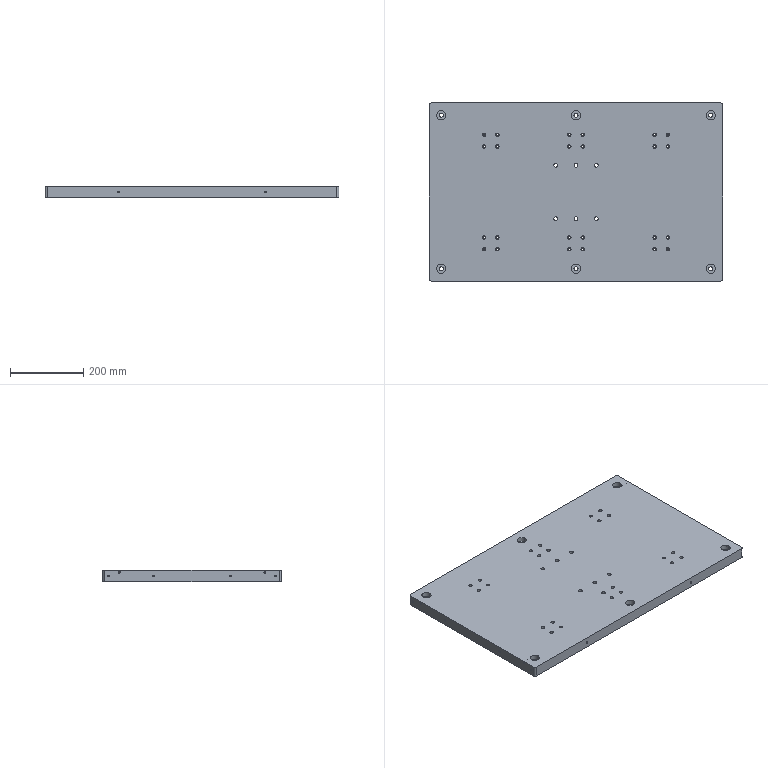NC program | Mastercam | posted with a generic post | part box 800 x 485 x 30 mm
Lines 3325 to 4968 of 13355:
N3520 T9 M6
N3530 G0 G90 G17 G54 X281.048 Y74.555 A0. S7000 M3
N3540 G43 H9 Z50. M8
N3550 Z1.
N3560 G1 Z-1.738 F600.
N3570 X280.896 Y75.543 F3000.
N3580 G3 X279.908 Y76.391 I-.988 J-.152
N3590 X279.756 Y76.379 I0. J-1.
N3600 G1 X273.1 Y75.355
N3610 Y69.122
N3620 G3 X274.1 Y68.122 I1. J0.
N3630 G1 X275.1
N3640 X281.048 Y74.555
N3650 Z-3.475 F600.
N3660 X280.896 Y75.543 F3000.
N3670 G3 X279.908 Y76.391 I-.988 J-.152
N3680 X279.756 Y76.379 I0. J-1.
N3690 G1 X273.1 Y75.355
N3700 Y69.122
N3710 G3 X274.1 Y68.122 I1. J0.
N3720 G1 X275.1
N3730 X281.048 Y74.555
N3740 Z-5.213 F600.
N3750 X280.896 Y75.543 F3000.
N3760 G3 X279.908 Y76.391 I-.988 J-.152
N3770 X279.756 Y76.379 I0. J-1.
N3780 G1 X273.1 Y75.355
N3790 Y69.122
N3800 G3 X274.1 Y68.122 I1. J0.
N3810 G1 X275.1
N3820 X281.048 Y74.555
N3830 Z-6.95 F600.
N3840 X280.896 Y75.543 F3000.
N3850 G3 X279.908 Y76.391 I-.988 J-.152
N3860 X279.756 Y76.379 I0. J-1.
N3870 G1 X273.1 Y75.355
N3880 Y69.122
N3890 G3 X274.1 Y68.122 I1. J0.
N3900 G1 X275.1
N3910 G0 Z50.
N3920 Y-75.399
N3930 Z1.
N3940 G1 Z-1.738 F600.
N3950 X274.1 F3000.
N3960 G3 X273.1 Y-76.399 I0. J-1.
N3970 G1 Y-83.4
N3980 X280.282
N3990 G3 X281.282 Y-82.4 I0. J1.
N4000 G1 Y-81.4
N4010 X275.1 Y-75.399
N4020 Z-3.475 F600.
N4030 X274.1 F3000.
N4040 G3 X273.1 Y-76.399 I0. J-1.
N4050 G1 Y-83.4
N4060 X280.282
N4070 G3 X281.282 Y-82.4 I0. J1.
N4080 G1 Y-81.4
N4090 X275.1 Y-75.399
N4100 Z-5.213 F600.
N4110 X274.1 F3000.
N4120 G3 X273.1 Y-76.399 I0. J-1.
N4130 G1 Y-83.4
N4140 X280.282
N4150 G3 X281.282 Y-82.4 I0. J1.
N4160 G1 Y-81.4
N4170 X275.1 Y-75.399
N4180 Z-6.95 F600.
N4190 X274.1 F3000.
N4200 G3 X273.1 Y-76.399 I0. J-1.
N4210 G1 Y-83.4
N4220 X280.282
N4230 G3 X281.282 Y-82.4 I0. J1.
N4240 G1 Y-81.4
N4250 G0 Z50.
N4260 X368.741
N4270 Z1.
N4280 G1 Z-1.738 F600.
N4290 Y-82.4 F3000.
N4300 G3 X369.741 Y-83.4 I1. J0.
N4310 G1 X376.9
N4320 Y-76.373
N4330 G3 X375.9 Y-75.373 I-1. J0.
N4340 G1 X374.9
N4350 X368.741 Y-81.4
N4360 Z-3.475 F600.
N4370 Y-82.4 F3000.
N4380 G3 X369.741 Y-83.4 I1. J0.
N4390 G1 X376.9
N4400 Y-76.373
N4410 G3 X375.9 Y-75.373 I-1. J0.
N4420 G1 X374.9
N4430 X368.741 Y-81.4
N4440 Z-5.213 F600.
N4450 Y-82.4 F3000.
N4460 G3 X369.741 Y-83.4 I1. J0.
N4470 G1 X376.9
N4480 Y-76.373
N4490 G3 X375.9 Y-75.373 I-1. J0.
N4500 G1 X374.9
N4510 X368.741 Y-81.4
N4520 Z-6.95 F600.
N4530 Y-82.4 F3000.
N4540 G3 X369.741 Y-83.4 I1. J0.
N4550 G1 X376.9
N4560 Y-76.373
N4570 G3 X375.9 Y-75.373 I-1. J0.
N4580 G1 X374.9
N4590 G0 Z50.
N4600 Y68.162
N4610 Z1.
N4620 G1 Z-1.738 F600.
N4630 X375.9 F3000.
N4640 G3 X376.9 Y69.162 I0. J1.
N4650 G1 Y75.355
N4660 X370.266 Y76.376
N4670 G3 X370.114 Y76.388 I-.152 J-.988
N4680 X369.126 Y75.54 I0. J-1.
N4690 G1 X368.974 Y74.551
N4700 X374.9 Y68.162
N4710 Z-3.475 F600.
N4720 X375.9 F3000.
N4730 G3 X376.9 Y69.162 I0. J1.
N4740 G1 Y75.355
N4750 X370.266 Y76.376
N4760 G3 X370.114 Y76.388 I-.152 J-.988
N4770 X369.126 Y75.54 I0. J-1.
N4780 G1 X368.974 Y74.551
N4790 X374.9 Y68.162
N4800 Z-5.213 F600.
N4810 X375.9 F3000.
N4820 G3 X376.9 Y69.162 I0. J1.
N4830 G1 Y75.355
N4840 X370.266 Y76.376
N4850 G3 X370.114 Y76.388 I-.152 J-.988
N4860 X369.126 Y75.54 I0. J-1.
N4870 G1 X368.974 Y74.551
N4880 X374.9 Y68.162
N4890 Z-6.95 F600.
N4900 X375.9 F3000.
N4910 G3 X376.9 Y69.162 I0. J1.
N4920 G1 Y75.355
N4930 X370.266 Y76.376
N4940 G3 X370.114 Y76.388 I-.152 J-.988
N4950 X369.126 Y75.54 I0. J-1.
N4960 G1 X368.974 Y74.551
N4970 G0 Z50.
N4980 X151.048 Y74.555
N4990 Z1.
N5000 G1 Z-1.738 F600.
N5010 X150.896 Y75.543 F3000.
N5020 G3 X149.908 Y76.391 I-.988 J-.152
N5030 X149.756 Y76.379 I0. J-1.
N5040 G1 X143.1 Y75.355
N5050 Y69.122
N5060 G3 X144.1 Y68.122 I1. J0.
N5070 G1 X145.1
N5080 X151.048 Y74.555
N5090 Z-3.475 F600.
N5100 X150.896 Y75.543 F3000.
N5110 G3 X149.908 Y76.391 I-.988 J-.152
N5120 X149.756 Y76.379 I0. J-1.
N5130 G1 X143.1 Y75.355
N5140 Y69.122
N5150 G3 X144.1 Y68.122 I1. J0.
N5160 G1 X145.1
N5170 X151.048 Y74.555
N5180 Z-5.213 F600.
N5190 X150.896 Y75.543 F3000.
N5200 G3 X149.908 Y76.391 I-.988 J-.152
N5210 X149.756 Y76.379 I0. J-1.
N5220 G1 X143.1 Y75.355
N5230 Y69.122
N5240 G3 X144.1 Y68.122 I1. J0.
N5250 G1 X145.1
N5260 X151.048 Y74.555
N5270 Z-6.95 F600.
N5280 X150.896 Y75.543 F3000.
N5290 G3 X149.908 Y76.391 I-.988 J-.152
N5300 X149.756 Y76.379 I0. J-1.
N5310 G1 X143.1 Y75.355
N5320 Y69.122
N5330 G3 X144.1 Y68.122 I1. J0.
N5340 G1 X145.1
N5350 G0 Z50.
N5360 Y-75.399
N5370 Z1.
N5380 G1 Z-1.738 F600.
N5390 X144.1 F3000.
N5400 G3 X143.1 Y-76.399 I0. J-1.
N5410 G1 Y-83.4
N5420 X150.282
N5430 G3 X151.282 Y-82.4 I0. J1.
N5440 G1 Y-81.4
N5450 X145.1 Y-75.399
N5460 Z-3.475 F600.
N5470 X144.1 F3000.
N5480 G3 X143.1 Y-76.399 I0. J-1.
N5490 G1 Y-83.4
N5500 X150.282
N5510 G3 X151.282 Y-82.4 I0. J1.
N5520 G1 Y-81.4
N5530 X145.1 Y-75.399
N5540 Z-5.213 F600.
N5550 X144.1 F3000.
N5560 G3 X143.1 Y-76.399 I0. J-1.
N5570 G1 Y-83.4
N5580 X150.282
N5590 G3 X151.282 Y-82.4 I0. J1.
N5600 G1 Y-81.4
N5610 X145.1 Y-75.399
N5620 Z-6.95 F600.
N5630 X144.1 F3000.
N5640 G3 X143.1 Y-76.399 I0. J-1.
N5650 G1 Y-83.4
N5660 X150.282
N5670 G3 X151.282 Y-82.4 I0. J1.
N5680 G1 Y-81.4
N5690 G0 Z50.
N5700 X238.694
N5710 Z1.
N5720 G1 Z-1.738 F600.
N5730 Y-82.4 F3000.
N5740 G3 X239.694 Y-83.4 I1. J0.
N5750 G1 X246.9
N5760 Y-76.373
N5770 G3 X245.9 Y-75.373 I-1. J0.
N5780 G1 X244.9
N5790 X238.694 Y-81.4
N5800 Z-3.475 F600.
N5810 Y-82.4 F3000.
N5820 G3 X239.694 Y-83.4 I1. J0.
N5830 G1 X246.9
N5840 Y-76.373
N5850 G3 X245.9 Y-75.373 I-1. J0.
N5860 G1 X244.9
N5870 X238.694 Y-81.4
N5880 Z-5.213 F600.
N5890 Y-82.4 F3000.
N5900 G3 X239.694 Y-83.4 I1. J0.
N5910 G1 X246.9
N5920 Y-76.373
N5930 G3 X245.9 Y-75.373 I-1. J0.
N5940 G1 X244.9
N5950 X238.694 Y-81.4
N5960 Z-6.95 F600.
N5970 Y-82.4 F3000.
N5980 G3 X239.694 Y-83.4 I1. J0.
N5990 G1 X246.9
N6000 Y-76.373
N6010 G3 X245.9 Y-75.373 I-1. J0.
N6020 G1 X244.9
N6030 G0 Z50.
N6040 Y68.163
N6050 Z1.
N6060 G1 Z-1.738 F600.
N6070 X245.9 F3000.
N6080 G3 X246.9 Y69.163 I0. J1.
N6090 G1 Y75.355
N6100 X240.266 Y76.376
N6110 G3 X240.114 Y76.388 I-.152 J-.988
N6120 X239.126 Y75.54 I0. J-1.
N6130 G1 X238.974 Y74.551
N6140 X244.9 Y68.163
N6150 Z-3.475 F600.
N6160 X245.9 F3000.
N6170 G3 X246.9 Y69.163 I0. J1.
N6180 G1 Y75.355
N6190 X240.266 Y76.376
N6200 G3 X240.114 Y76.388 I-.152 J-.988
N6210 X239.126 Y75.54 I0. J-1.
N6220 G1 X238.974 Y74.551
N6230 X244.9 Y68.163
N6240 Z-5.213 F600.
N6250 X245.9 F3000.
N6260 G3 X246.9 Y69.163 I0. J1.
N6270 G1 Y75.355
N6280 X240.266 Y76.376
N6290 G3 X240.114 Y76.388 I-.152 J-.988
N6300 X239.126 Y75.54 I0. J-1.
N6310 G1 X238.974 Y74.551
N6320 X244.9 Y68.163
N6330 Z-6.95 F600.
N6340 X245.9 F3000.
N6350 G3 X246.9 Y69.163 I0. J1.
N6360 G1 Y75.355
N6370 X240.266 Y76.376
N6380 G3 X240.114 Y76.388 I-.152 J-.988
N6390 X239.126 Y75.54 I0. J-1.
N6400 G1 X238.974 Y74.551
N6410 G0 Z50.
N6420 X21.048 Y74.555
N6430 Z1.
N6440 G1 Z-1.738 F600.
N6450 X20.896 Y75.543 F3000.
N6460 G3 X19.908 Y76.391 I-.988 J-.152
N6470 X19.756 Y76.379 I0. J-1.
N6480 G1 X13.1 Y75.355
N6490 Y69.122
N6500 G3 X14.1 Y68.122 I1. J0.
N6510 G1 X15.1
N6520 X21.048 Y74.555
N6530 Z-3.475 F600.
N6540 X20.896 Y75.543 F3000.
N6550 G3 X19.908 Y76.391 I-.988 J-.152
N6560 X19.756 Y76.379 I0. J-1.
N6570 G1 X13.1 Y75.355
N6580 Y69.122
N6590 G3 X14.1 Y68.122 I1. J0.
N6600 G1 X15.1
N6610 X21.048 Y74.555
N6620 Z-5.213 F600.
N6630 X20.896 Y75.543 F3000.
N6640 G3 X19.908 Y76.391 I-.988 J-.152
N6650 X19.756 Y76.379 I0. J-1.
N6660 G1 X13.1 Y75.355
N6670 Y69.122
N6680 G3 X14.1 Y68.122 I1. J0.
N6690 G1 X15.1
N6700 X21.048 Y74.555
N6710 Z-6.95 F600.
N6720 X20.896 Y75.543 F3000.
N6730 G3 X19.908 Y76.391 I-.988 J-.152
N6740 X19.756 Y76.379 I0. J-1.
N6750 G1 X13.1 Y75.355
N6760 Y69.122
N6770 G3 X14.1 Y68.122 I1. J0.
N6780 G1 X15.1
N6790 G0 Z50.
N6800 Y-75.399
N6810 Z1.
N6820 G1 Z-1.738 F600.
N6830 X14.1 F3000.
N6840 G3 X13.1 Y-76.399 I0. J-1.
N6850 G1 Y-83.4
N6860 X20.282
N6870 G3 X21.282 Y-82.4 I0. J1.
N6880 G1 Y-81.4
N6890 X15.1 Y-75.399
N6900 Z-3.475 F600.
N6910 X14.1 F3000.
N6920 G3 X13.1 Y-76.399 I0. J-1.
N6930 G1 Y-83.4
N6940 X20.282
N6950 G3 X21.282 Y-82.4 I0. J1.
N6960 G1 Y-81.4
N6970 X15.1 Y-75.399
N6980 Z-5.213 F600.
N6990 X14.1 F3000.
N7000 G3 X13.1 Y-76.399 I0. J-1.
N7010 G1 Y-83.4
N7020 X20.282
N7030 G3 X21.282 Y-82.4 I0. J1.
N7040 G1 Y-81.4
N7050 X15.1 Y-75.399
N7060 Z-6.95 F600.
N7070 X14.1 F3000.
N7080 G3 X13.1 Y-76.399 I0. J-1.
N7090 G1 Y-83.4
N7100 X20.282
N7110 G3 X21.282 Y-82.4 I0. J1.
N7120 G1 Y-81.4
N7130 G0 Z50.
N7140 X108.744
N7150 Z1.
N7160 G1 Z-1.738 F600.
N7170 Y-82.4 F3000.
N7180 G3 X109.744 Y-83.4 I1. J0.
N7190 G1 X116.9
N7200 Y-76.373
N7210 G3 X115.9 Y-75.373 I-1. J0.
N7220 G1 X114.9
N7230 X108.744 Y-81.4
N7240 Z-3.475 F600.
N7250 Y-82.4 F3000.
N7260 G3 X109.744 Y-83.4 I1. J0.
N7270 G1 X116.9
N7280 Y-76.373
N7290 G3 X115.9 Y-75.373 I-1. J0.
N7300 G1 X114.9
N7310 X108.744 Y-81.4
N7320 Z-5.213 F600.
N7330 Y-82.4 F3000.
N7340 G3 X109.744 Y-83.4 I1. J0.
N7350 G1 X116.9
N7360 Y-76.373
N7370 G3 X115.9 Y-75.373 I-1. J0.
N7380 G1 X114.9
N7390 X108.744 Y-81.4
N7400 Z-6.95 F600.
N7410 Y-82.4 F3000.
N7420 G3 X109.744 Y-83.4 I1. J0.
N7430 G1 X116.9
N7440 Y-76.373
N7450 G3 X115.9 Y-75.373 I-1. J0.
N7460 G1 X114.9
N7470 G0 Z50.
N7480 Y68.106
N7490 Z1.
N7500 G1 Z-1.738 F600.
N7510 X115.9 F3000.
N7520 G3 X116.9 Y69.106 I0. J1.
N7530 G1 Y75.355
N7540 X110.266 Y76.376
N7550 G3 X110.114 Y76.388 I-.152 J-.988
N7560 X109.126 Y75.54 I0. J-1.
N7570 G1 X108.974 Y74.551
N7580 X114.9 Y68.106
N7590 Z-3.475 F600.
N7600 X115.9 F3000.
N7610 G3 X116.9 Y69.106 I0. J1.
N7620 G1 Y75.355
N7630 X110.266 Y76.376
N7640 G3 X110.114 Y76.388 I-.152 J-.988
N7650 X109.126 Y75.54 I0. J-1.
N7660 G1 X108.974 Y74.551
N7670 X114.9 Y68.106
N7680 Z-5.213 F600.
N7690 X115.9 F3000.
N7700 G3 X116.9 Y69.106 I0. J1.
N7710 G1 Y75.355
N7720 X110.266 Y76.376
N7730 G3 X110.114 Y76.388 I-.152 J-.988
N7740 X109.126 Y75.54 I0. J-1.
N7750 G1 X108.974 Y74.551
N7760 X114.9 Y68.106
N7770 Z-6.95 F600.
N7780 X115.9 F3000.
N7790 G3 X116.9 Y69.106 I0. J1.
N7800 G1 Y75.355
N7810 X110.266 Y76.376
N7820 G3 X110.114 Y76.388 I-.152 J-.988
N7830 X109.126 Y75.54 I0. J-1.
N7840 G1 X108.974 Y74.551
N7850 G0 Z50.
N7860 X-238.952 Y74.555
N7870 Z1.
N7880 G1 Z-1.738 F600.
N7890 X-239.104 Y75.543 F3000.
N7900 G3 X-240.092 Y76.391 I-.988 J-.152
N7910 X-240.244 Y76.379 I0. J-1.
N7920 G1 X-246.9 Y75.355
N7930 Y69.122
N7940 G3 X-245.9 Y68.122 I1. J0.
N7950 G1 X-244.9
N7960 X-238.952 Y74.555
N7970 Z-3.475 F600.
N7980 X-239.104 Y75.543 F3000.
N7990 G3 X-240.092 Y76.391 I-.988 J-.152
N8000 X-240.244 Y76.379 I0. J-1.
N8010 G1 X-246.9 Y75.355
N8020 Y69.122
N8030 G3 X-245.9 Y68.122 I1. J0.
N8040 G1 X-244.9
N8050 X-238.952 Y74.555
N8060 Z-5.213 F600.
N8070 X-239.104 Y75.543 F3000.
N8080 G3 X-240.092 Y76.391 I-.988 J-.152
N8090 X-240.244 Y76.379 I0. J-1.
N8100 G1 X-246.9 Y75.355
N8110 Y69.122
N8120 G3 X-245.9 Y68.122 I1. J0.
N8130 G1 X-244.9
N8140 X-238.952 Y74.555
N8150 Z-6.95 F600.
N8160 X-239.104 Y75.543 F3000.
N8170 G3 X-240.092 Y76.391 I-.988 J-.152
N8180 X-240.244 Y76.379 I0. J-1.
N8190 G1 X-246.9 Y75.355
N8200 Y69.122
N8210 G3 X-245.9 Y68.122 I1. J0.
N8220 G1 X-244.9
N8230 G0 Z50.
N8240 Y-75.399
N8250 Z1.
N8260 G1 Z-1.738 F600.
N8270 X-245.9 F3000.
N8280 G3 X-246.9 Y-76.399 I0. J-1.
N8290 G1 Y-83.4
N8300 X-239.718
N8310 G3 X-238.718 Y-82.4 I0. J1.
N8320 G1 Y-81.4
N8330 X-244.9 Y-75.399
N8340 Z-3.475 F600.
N8350 X-245.9 F3000.
N8360 G3 X-246.9 Y-76.399 I0. J-1.
N8370 G1 Y-83.4
N8380 X-239.718
N8390 G3 X-238.718 Y-82.4 I0. J1.
N8400 G1 Y-81.4
N8410 X-244.9 Y-75.399
N8420 Z-5.213 F600.
N8430 X-245.9 F3000.
N8440 G3 X-246.9 Y-76.399 I0. J-1.
N8450 G1 Y-83.4
N8460 X-239.718
N8470 G3 X-238.718 Y-82.4 I0. J1.
N8480 G1 Y-81.4
N8490 X-244.9 Y-75.399
N8500 Z-6.95 F600.
N8510 X-245.9 F3000.
N8520 G3 X-246.9 Y-76.399 I0. J-1.
N8530 G1 Y-83.4
N8540 X-239.718
N8550 G3 X-238.718 Y-82.4 I0. J1.
N8560 G1 Y-81.4
N8570 G0 Z50.
N8580 X-151.306
N8590 Z1.
N8600 G1 Z-1.738 F600.
N8610 Y-82.4 F3000.
N8620 G3 X-150.306 Y-83.4 I1. J0.
N8630 G1 X-143.1
N8640 Y-76.373
N8650 G3 X-144.1 Y-75.373 I-1. J0.
N8660 G1 X-145.1
N8670 X-151.306 Y-81.4
N8680 Z-3.475 F600.
N8690 Y-82.4 F3000.
N8700 G3 X-150.306 Y-83.4 I1. J0.
N8710 G1 X-143.1
N8720 Y-76.373
N8730 G3 X-144.1 Y-75.373 I-1. J0.
N8740 G1 X-145.1
N8750 X-151.306 Y-81.4
N8760 Z-5.213 F600.
N8770 Y-82.4 F3000.
N8780 G3 X-150.306 Y-83.4 I1. J0.
N8790 G1 X-143.1
N8800 Y-76.373
N8810 G3 X-144.1 Y-75.373 I-1. J0.
N8820 G1 X-145.1
N8830 X-151.306 Y-81.4
N8840 Z-6.95 F600.
N8850 Y-82.4 F3000.
N8860 G3 X-150.306 Y-83.4 I1. J0.
N8870 G1 X-143.1
N8880 Y-76.373
N8890 G3 X-144.1 Y-75.373 I-1. J0.
N8900 G1 X-145.1
N8910 G0 Z50.
N8920 Y68.163
N8930 Z1.
N8940 G1 Z-1.738 F600.
N8950 X-144.1 F3000.
N8960 G3 X-143.1 Y69.163 I0. J1.
N8970 G1 Y75.355
N8980 X-149.734 Y76.376
N8990 G3 X-149.886 Y76.388 I-.152 J-.988
N9000 X-150.874 Y75.54 I0. J-1.
N9010 G1 X-151.026 Y74.551
N9020 X-145.1 Y68.163
N9030 Z-3.475 F600.
N9040 X-144.1 F3000.
N9050 G3 X-143.1 Y69.163 I0. J1.
N9060 G1 Y75.355
N9070 X-149.734 Y76.376
N9080 G3 X-149.886 Y76.388 I-.152 J-.988
N9090 X-150.874 Y75.54 I0. J-1.
N9100 G1 X-151.026 Y74.551
N9110 X-145.1 Y68.163
N9120 Z-5.213 F600.
N9130 X-144.1 F3000.
N9140 G3 X-143.1 Y69.163 I0. J1.
N9150 G1 Y75.355
N9160 X-149.734 Y76.376
N9170 G3 X-149.886 Y76.388 I-.152 J-.988
N9180 X-150.874 Y75.54 I0. J-1.
N9190 G1 X-151.026 Y74.551
N9200 X-145.1 Y68.163
N9210 Z-6.95 F600.
N9220 X-144.1 F3000.
N9230 G3 X-143.1 Y69.163 I0. J1.
N9240 G1 Y75.355
N9250 X-149.734 Y76.376
N9260 G3 X-149.886 Y76.388 I-.152 J-.988
N9270 X-150.874 Y75.54 I0. J-1.
N9280 G1 X-151.026 Y74.551
N9290 G0 Z50.
N9300 X-321.94 Y80.846
N9310 Z1.
N9320 G1 Z-1.738 F600.
N9330 X-321.788 Y81.834 F3000.
N9340 G3 X-321.776 Y81.986 I-.988 J.152
N9350 X-322.624 Y82.975 I-1. J0.
N9360 G1 X-325. Y83.34
N9370 X-328.29 Y82.834
N9380 G3 X-329.137 Y81.846 I.153 J-.988
N9390 X-329.126 Y81.693 I1. J0.
N9400 G1 X-328.974 Y80.705
N9410 X-321.94 Y80.846
N9420 Z-3.475 F600.
N9430 X-321.788 Y81.834 F3000.
N9440 G3 X-321.776 Y81.986 I-.988 J.152
N9450 X-322.624 Y82.975 I-1. J0.
N9460 G1 X-325. Y83.34
N9470 X-328.29 Y82.834
N9480 G3 X-329.137 Y81.846 I.153 J-.988
N9490 X-329.126 Y81.693 I1. J0.
N9500 G1 X-328.974 Y80.705
N9510 X-321.94 Y80.846
N9520 Z-5.213 F600.
N9530 X-321.788 Y81.834 F3000.
N9540 G3 X-321.776 Y81.986 I-.988 J.152
N9550 X-322.624 Y82.975 I-1. J0.
N9560 G1 X-325. Y83.34
N9570 X-328.29 Y82.834
N9580 G3 X-329.137 Y81.846 I.153 J-.988
N9590 X-329.126 Y81.693 I1. J0.
N9600 G1 X-328.974 Y80.705
N9610 X-321.94 Y80.846
N9620 Z-6.95 F600.
N9630 X-321.788 Y81.834 F3000.
N9640 G3 X-321.776 Y81.986 I-.988 J.152
N9650 X-322.624 Y82.975 I-1. J0.
N9660 G1 X-325. Y83.34
N9670 X-328.29 Y82.834
N9680 G3 X-329.137 Y81.846 I.153 J-.988
N9690 X-329.126 Y81.693 I1. J0.
N9700 G1 X-328.974 Y80.705
N9710 G0 Z50.
N9720 X-368.952 Y74.555
N9730 Z1.
N9740 G1 Z-1.738 F600.
N9750 X-369.104 Y75.543 F3000.
N9760 G3 X-370.092 Y76.391 I-.988 J-.152
N9770 X-370.244 Y76.379 I0. J-1.
N9780 G1 X-376.9 Y75.355
N9790 Y69.122
N9800 G3 X-375.9 Y68.122 I1. J0.
N9810 G1 X-374.9
N9820 X-368.952 Y74.555
N9830 Z-3.475 F600.
N9840 X-369.104 Y75.543 F3000.
N9850 G3 X-370.092 Y76.391 I-.988 J-.152
N9860 X-370.244 Y76.379 I0. J-1.
N9870 G1 X-376.9 Y75.355
N9880 Y69.122
N9890 G3 X-375.9 Y68.122 I1. J0.
N9900 G1 X-374.9
N9910 X-368.952 Y74.555
N9920 Z-5.213 F600.
N9930 X-369.104 Y75.543 F3000.
N9940 G3 X-370.092 Y76.391 I-.988 J-.152
N9950 X-370.244 Y76.379 I0. J-1.
N9960 G1 X-376.9 Y75.355
N9970 Y69.122
N9980 G3 X-375.9 Y68.122 I1. J0.
N9990 G1 X-374.9
N100 X-368.952 Y74.555
N110 Z-6.95 F600.
N120 X-369.104 Y75.543 F3000.
N130 G3 X-370.092 Y76.391 I-.988 J-.152
N140 X-370.244 Y76.379 I0. J-1.
N150 G1 X-376.9 Y75.355
N160 Y69.122
N170 G3 X-375.9 Y68.122 I1. J0.
N180 G1 X-374.9
N190 G0 Z50.
N200 Y-75.399
N210 Z1.
N220 G1 Z-1.738 F600.
N230 X-375.9 F3000.
N240 G3 X-376.9 Y-76.399 I0. J-1.
N250 G1 Y-83.4
N260 X-369.718
N270 G3 X-368.718 Y-82.4 I0. J1.
N280 G1 Y-81.4
N290 X-374.9 Y-75.399
N300 Z-3.475 F600.
N310 X-375.9 F3000.
N320 G3 X-376.9 Y-76.399 I0. J-1.
N330 G1 Y-83.4
N340 X-369.718
N350 G3 X-368.718 Y-82.4 I0. J1.
N360 G1 Y-81.4
N370 X-374.9 Y-75.399
N380 Z-5.213 F600.
N390 X-375.9 F3000.
N400 G3 X-376.9 Y-76.399 I0. J-1.
N410 G1 Y-83.4
N420 X-369.718
N430 G3 X-368.718 Y-82.4 I0. J1.
N440 G1 Y-81.4
N450 X-374.9 Y-75.399
N460 Z-6.95 F600.
N470 X-375.9 F3000.
N480 G3 X-376.9 Y-76.399 I0. J-1.
N490 G1 Y-83.4
N500 X-369.718
N510 G3 X-368.718 Y-82.4 I0. J1.
N520 G1 Y-81.4
N530 G0 Z50.
N540 X-281.256
N550 Z1.
N560 G1 Z-1.738 F600.
N570 Y-82.4 F3000.
N580 G3 X-280.256 Y-83.4 I1. J0.
N590 G1 X-273.1
N600 Y-76.373
N610 G3 X-274.1 Y-75.373 I-1. J0.
N620 G1 X-275.1
N630 X-281.256 Y-81.4
N640 Z-3.475 F600.
N650 Y-82.4 F3000.
N660 G3 X-280.256 Y-83.4 I1. J0.
N670 G1 X-273.1
N680 Y-76.373
N690 G3 X-274.1 Y-75.373 I-1. J0.
N700 G1 X-275.1
N710 X-281.256 Y-81.4
N720 Z-5.213 F600.
N730 Y-82.4 F3000.
N740 G3 X-280.256 Y-83.4 I1. J0.
N750 G1 X-273.1
N760 Y-76.373
N770 G3 X-274.1 Y-75.373 I-1. J0.
N780 G1 X-275.1
N790 X-281.256 Y-81.4
N800 Z-6.95 F600.
N810 Y-82.4 F3000.
N820 G3 X-280.256 Y-83.4 I1. J0.
N830 G1 X-273.1
N840 Y-76.373
N850 G3 X-274.1 Y-75.373 I-1. J0.
N860 G1 X-275.1
N870 G0 Z50.
N880 Y68.122
N890 Z1.
N900 G1 Z-1.738 F600.
N910 X-274.1 F3000.
N920 G3 X-273.1 Y69.122 I0. J1.
N930 G1 Y75.355
N940 X-279.734 Y76.376
N950 G3 X-279.886 Y76.388 I-.152 J-.988
N960 X-280.874 Y75.54 I0. J-1.
N970 G1 X-281.026 Y74.551
N980 X-275.1 Y68.122
N990 Z-3.475 F600.
N1000 X-274.1 F3000.
N1010 G3 X-273.1 Y69.122 I0. J1.
N1020 G1 Y75.355
N1030 X-279.734 Y76.376
N1040 G3 X-279.886 Y76.388 I-.152 J-.988
N1050 X-280.874 Y75.54 I0. J-1.
N1060 G1 X-281.026 Y74.551
N1070 X-275.1 Y68.122
N1080 Z-5.213 F600.
N1090 X-274.1 F3000.
N1100 G3 X-273.1 Y69.122 I0. J1.
N1110 G1 Y75.355
N1120 X-279.734 Y76.376
N1130 G3 X-279.886 Y76.388 I-.152 J-.988
N1140 X-280.874 Y75.54 I0. J-1.
N1150 G1 X-281.026 Y74.551
N1160 X-275.1 Y68.122
N1170 Z-6.95 F600.
N1180 X-274.1 F3000.
N1190 G3 X-273.1 Y69.122 I0. J1.
N1200 G1 Y75.355
N1210 X-279.734 Y76.376
N1220 G3 X-279.886 Y76.388 I-.152 J-.988
N1230 X-280.874 Y75.54 I0. J-1.
N1240 G1 X-281.026 Y74.551
N1250 G0 Z50.
N1260 X-108.952 Y74.555
N1270 Z1.
N1280 G1 Z-1.738 F600.
N1290 X-109.104 Y75.543 F3000.
N1300 G3 X-110.092 Y76.391 I-.988 J-.152
N1310 X-110.244 Y76.379 I0. J-1.
N1320 G1 X-116.9 Y75.355
N1330 Y69.122
N1340 G3 X-115.9 Y68.122 I1. J0.
N1350 G1 X-114.9
N1360 X-108.952 Y74.555
N1370 Z-3.475 F600.
N1380 X-109.104 Y75.543 F3000.
N1390 G3 X-110.092 Y76.391 I-.988 J-.152
N1400 X-110.244 Y76.379 I0. J-1.
N1410 G1 X-116.9 Y75.355
N1420 Y69.122
N1430 G3 X-115.9 Y68.122 I1. J0.
N1440 G1 X-114.9
N1450 X-108.952 Y74.555
N1460 Z-5.213 F600.
N1470 X-109.104 Y75.543 F3000.
N1480 G3 X-110.092 Y76.391 I-.988 J-.152
N1490 X-110.244 Y76.379 I0. J-1.
N1500 G1 X-116.9 Y75.355
N1510 Y69.122
N1520 G3 X-115.9 Y68.122 I1. J0.
N1530 G1 X-114.9
N1540 X-108.952 Y74.555
N1550 Z-6.95 F600.
N1560 X-109.104 Y75.543 F3000.
N1570 G3 X-110.092 Y76.391 I-.988 J-.152
N1580 X-110.244 Y76.379 I0. J-1.
N1590 G1 X-116.9 Y75.355
N1600 Y69.122
N1610 G3 X-115.9 Y68.122 I1. J0.
N1620 G1 X-114.9
N1630 G0 Z50.
N1640 Y-75.399
N1650 Z1.
N1660 G1 Z-1.738 F600.
N1670 X-115.9 F3000.
N1680 G3 X-116.9 Y-76.399 I0. J-1.
N1690 G1 Y-83.4
N1700 X-109.718
N1710 G3 X-108.718 Y-82.4 I0. J1.
N1720 G1 Y-81.4
N1730 X-114.9 Y-75.399
N1740 Z-3.475 F600.
N1750 X-115.9 F3000.
N1760 G3 X-116.9 Y-76.399 I0. J-1.
N1770 G1 Y-83.4
N1780 X-109.718
N1790 G3 X-108.718 Y-82.4 I0. J1.
N1800 G1 Y-81.4
N1810 X-114.9 Y-75.399
N1820 Z-5.213 F600.
N1830 X-115.9 F3000.
N1840 G3 X-116.9 Y-76.399 I0. J-1.
N1850 G1 Y-83.4
N1860 X-109.718
N1870 G3 X-108.718 Y-82.4 I0. J1.
N1880 G1 Y-81.4
N1890 X-114.9 Y-75.399
N1900 Z-6.95 F600.
N1910 X-115.9 F3000.
N1920 G3 X-116.9 Y-76.399 I0. J-1.
N1930 G1 Y-83.4
N1940 X-109.718
N1950 G3 X-108.718 Y-82.4 I0. J1.
N1960 G1 Y-81.4
N1970 G0 Z50.
N1980 X-21.256
N1990 Z1.
N2000 G1 Z-1.738 F600.
N2010 Y-82.4 F3000.
N2020 G3 X-20.256 Y-83.4 I1. J0.
N2030 G1 X-13.1
N2040 Y-76.373
N2050 G3 X-14.1 Y-75.373 I-1. J0.
N2060 G1 X-15.1
N2070 X-21.256 Y-81.4
N2080 Z-3.475 F600.
N2090 Y-82.4 F3000.
N2100 G3 X-20.256 Y-83.4 I1. J0.
N2110 G1 X-13.1
N2120 Y-76.373
N2130 G3 X-14.1 Y-75.373 I-1. J0.
N2140 G1 X-15.1
N2150 X-21.256 Y-81.4
N2160 Z-5.213 F600.
N2170 Y-82.4 F3000.
N2180 G3 X-20.256 Y-83.4 I1. J0.
N2190 G1 X-13.1
N2200 Y-76.373
N2210 G3 X-14.1 Y-75.373 I-1. J0.
N2220 G1 X-15.1
N2230 X-21.256 Y-81.4
N2240 Z-6.95 F600.
N2250 Y-82.4 F3000.
N2260 G3 X-20.256 Y-83.4 I1. J0.
N2270 G1 X-13.1
N2280 Y-76.373
N2290 G3 X-14.1 Y-75.373 I-1. J0.
N2300 G1 X-15.1
N2310 G0 Z50.
N2320 Y68.122
N2330 Z1.
N2340 G1 Z-1.738 F600.
N2350 X-14.1 F3000.
N2360 G3 X-13.1 Y69.122 I0. J1.
N2370 G1 Y75.355
N2380 X-19.734 Y76.376
N2390 G3 X-19.886 Y76.388 I-.152 J-.988
N2400 X-20.874 Y75.54 I0. J-1.
N2410 G1 X-21.026 Y74.551
N2420 X-15.1 Y68.122
N2430 Z-3.475 F600.
N2440 X-14.1 F3000.
N2450 G3 X-13.1 Y69.122 I0. J1.
N2460 G1 Y75.355
N2470 X-19.734 Y76.376
N2480 G3 X-19.886 Y76.388 I-.152 J-.988
N2490 X-20.874 Y75.54 I0. J-1.
N2500 G1 X-21.026 Y74.551
N2510 X-15.1 Y68.122
N2520 Z-5.213 F600.
N2530 X-14.1 F3000.
N2540 G3 X-13.1 Y69.122 I0. J1.
N2550 G1 Y75.355
N2560 X-19.734 Y76.376
N2570 G3 X-19.886 Y76.388 I-.152 J-.988
N2580 X-20.874 Y75.54 I0. J-1.
N2590 G1 X-21.026 Y74.551
N2600 X-15.1 Y68.122
N2610 Z-6.95 F600.
N2620 X-14.1 F3000.
N2630 G3 X-13.1 Y69.122 I0. J1.
N2640 G1 Y75.355
N2650 X-19.734 Y76.376
N2660 G3 X-19.886 Y76.388 I-.152 J-.988
N2670 X-20.874 Y75.54 I0. J-1.
N2680 G1 X-21.026 Y74.551
N2690 G0 Z50.
N2700 X-61.94 Y80.846
N2710 Z1.
N2720 G1 Z-1.738 F600.
N2730 X-61.788 Y81.834 F3000.
N2740 G3 X-61.776 Y81.986 I-.988 J.152
N2750 X-62.624 Y82.975 I-1. J0.
N2760 G1 X-65. Y83.34
N2770 X-68.29 Y82.834
N2780 G3 X-69.137 Y81.846 I.153 J-.988
N2790 X-69.126 Y81.693 I1. J0.
N2800 G1 X-68.974 Y80.705
N2810 X-61.94 Y80.846
N2820 Z-3.475 F600.
N2830 X-61.788 Y81.834 F3000.
N2840 G3 X-61.776 Y81.986 I-.988 J.152
N2850 X-62.624 Y82.975 I-1. J0.
N2860 G1 X-65. Y83.34
N2870 X-68.29 Y82.834
N2880 G3 X-69.137 Y81.846 I.153 J-.988
N2890 X-69.126 Y81.693 I1. J0.
N2900 G1 X-68.974 Y80.705
N2910 X-61.94 Y80.846
N2920 Z-5.213 F600.
N2930 X-61.788 Y81.834 F3000.
N2940 G3 X-61.776 Y81.986 I-.988 J.152
N2950 X-62.624 Y82.975 I-1. J0.
N2960 G1 X-65. Y83.34
N2970 X-68.29 Y82.834
N2980 G3 X-69.137 Y81.846 I.153 J-.988
N2990 X-69.126 Y81.693 I1. J0.
N3000 G1 X-68.974 Y80.705
N3010 X-61.94 Y80.846
N3020 Z-6.95 F600.
N3030 X-61.788 Y81.834 F3000.
N3040 G3 X-61.776 Y81.986 I-.988 J.152
N3050 X-62.624 Y82.975 I-1. J0.
N3060 G1 X-65. Y83.34
N3070 X-68.29 Y82.834
N3080 G3 X-69.137 Y81.846 I.153 J-.988
N3090 X-69.126 Y81.693 I1. J0.
N3100 G1 X-68.974 Y80.705
N3110 G0 Z50.
N3120 M5
N3130 G91 G28 Z0. M9
N3140 A0.
N3150 M01
N3160 T10 M6
N3170 G0 G90 G17 G54 X325. Y-7.851 A0. S7000 M3
N3180 G43 H10 Z50. M8
N3190 Z-6.
N3200 G1 Z-6.708 F600.
N3210 Y-2.351 Z-6.854 F1000.
N3220 Y-.335 Z-6.908
N3230 Y3.149 Z-7.
N3240 Y30.83
N3250 Y-31.5
N3260 Y-.335
N3270 Y3.149
N3280 G2 X325.805 Y4.155 I1.031 J0.
N3290 G1 X330.615 Y5.236
N3300 G3 X331.42 Y6.242 I-.226 J1.006
N3310 G1 Y36.337
N3320 X325. Y37.325
N3330 X318.58 Y36.337
N3340 Y-37.92
N3350 X331.42
N3360 Y-.335
N3370 Y6.242
N3380 G2 X332.229 Y7.249 I1.031 J0.
N3390 G1 X337.122 Y8.329
N3400 G3 X337.931 Y9.336 I-.222 J1.007
N3410 G1 Y41.923
N3420 X325. Y43.913
N3430 X312.069 Y41.923
N3440 Y-44.431
N3450 X337.931
N3460 Y-.335
N3470 Y9.336
N3480 G2 X338.74 Y10.343 I1.031 J0.
N3490 G1 X343.634 Y11.423
N3500 G3 X344.443 Y12.43 I-.223 J1.007
N3510 G1 Y47.51
N3520 X325. Y50.501
N3530 X305.557 Y47.51
N3540 Y-50.943
N3550 X344.443
N3560 Y-.335
N3570 Y12.43
N3580 G2 X345.252 Y13.437 I1.031 J0.
N3590 G1 X350.145 Y14.517
N3600 G3 X350.954 Y15.524 I-.222 J1.007
N3610 G1 Y53.096
N3620 X325. Y57.089
N3630 X299.046 Y53.096
N3640 Y-57.454
N3650 X350.954
N3660 Y-.335
N3670 Y15.524
N3680 G2 X351.763 Y16.531 I1.031 J0.
N3690 G1 X356.657 Y17.61
N3700 G3 X357.466 Y18.617 I-.223 J1.007
N3710 G1 Y58.682
N3720 X325. Y63.677
N3730 X292.534 Y58.682
N3740 Y-63.966
N3750 X357.466
N3760 Y-.335
N3770 Y18.617
N3780 G2 X358.275 Y19.624 I1.031 J0.
N3790 G1 X363.168 Y20.704
N3800 G3 X363.977 Y21.711 I-.222 J1.007
N3810 G1 Y64.269
N3820 X325. Y70.265
N3830 X286.023 Y64.269
N3840 Y-70.477
N3850 X363.977
N3860 Y-.335
N3870 Y21.711
N3880 G2 X364.786 Y22.718 I1.031 J0.
N3890 G1 X369.679 Y23.798
N3900 G3 X370.488 Y24.805 I-.222 J1.007
N3910 G1 Y69.855
N3920 X325. Y76.853
N3930 X279.512 Y69.855
N3940 Y-76.988
N3950 X370.488
N3960 Y-.335
N3970 Y24.805
N3980 G2 X371.297 Y25.812 I1.032 J0.
N3990 G1 X376.185 Y26.893
N4000 G3 X376.993 Y27.9 I-.223 J1.007
N4010 G1 X376.982 Y75.424
N4020 X325. Y83.427
N4030 X273.018 Y75.424
N4040 X273. Y75.084
N4050 Y-82.902
N4060 X273.022 Y-83.478
N4070 X273.523 Y-83.5
N4080 X376.477
N4090 X376.978 Y-83.478
N4100 X377. Y-82.902
N4110 Y-.335
N4120 X376.993 Y27.9
N4130 G0 Z50.
N4140 X195. Y-7.851
N4150 Z-6.
N4160 G1 Z-6.708 F600.
N4170 Y-2.351 Z-6.854 F1000.
N4180 Y-.335 Z-6.908
N4190 Y3.149 Z-7.
N4200 Y30.83
N4210 Y-31.5
N4220 Y-.335
N4230 Y3.149
N4240 G2 X195.805 Y4.155 I1.031 J0.
N4250 G1 X200.615 Y5.236
N4260 G3 X201.42 Y6.242 I-.226 J1.006
N4270 G1 Y36.337
N4280 X195. Y37.325
N4290 X188.58 Y36.337
N4300 Y-37.92
N4310 X201.42
N4320 Y-.335
N4330 Y6.242
N4340 G2 X202.229 Y7.249 I1.031 J0.
N4350 G1 X207.122 Y8.329
N4360 G3 X207.931 Y9.336 I-.222 J1.007
N4370 G1 Y41.923
N4380 X195. Y43.913
N4390 X182.069 Y41.923
N4400 Y-44.431
N4410 X207.931
N4420 Y-.335
N4430 Y9.336
N4440 G2 X208.74 Y10.343 I1.031 J0.
N4450 G1 X213.634 Y11.423
N4460 G3 X214.443 Y12.43 I-.223 J1.007
N4470 G1 Y47.51
N4480 X195. Y50.501
N4490 X175.557 Y47.51
N4500 Y-50.943
N4510 X214.443
N4520 Y-.335
N4530 Y12.43
N4540 G2 X215.252 Y13.437 I1.031 J0.
N4550 G1 X220.145 Y14.517
N4560 G3 X220.954 Y15.524 I-.222 J1.007
N4570 G1 Y53.096
N4580 X195. Y57.089
N4590 X169.046 Y53.096
N4600 Y-57.454
N4610 X220.954
N4620 Y-.335
N4630 Y15.524
N4640 G2 X221.763 Y16.531 I1.031 J0.
N4650 G1 X226.657 Y17.61
N4660 G3 X227.466 Y18.617 I-.223 J1.007
N4670 G1 Y58.682
N4680 X195. Y63.677
N4690 X162.534 Y58.682
N4700 Y-63.966
N4710 X227.466
N4720 Y-.335
N4730 Y18.617
N4740 G2 X228.275 Y19.624 I1.031 J0.
N4750 G1 X233.168 Y20.704
N4760 G3 X233.977 Y21.711 I-.222 J1.007
N4770 G1 Y64.269
N4780 X195. Y70.265
N4790 X156.023 Y64.269
N4800 Y-70.477
N4810 X233.977
N4820 Y-.335
N4830 Y21.711
N4840 G2 X234.786 Y22.718 I1.031 J0.
N4850 G1 X239.679 Y23.798
N4860 G3 X240.488 Y24.805 I-.222 J1.007
N4870 G1 Y69.855
N4880 X195. Y76.853
N4890 X149.512 Y69.855
N4900 Y-76.988
N4910 X240.488
N4920 Y-.335
N4930 Y24.805
N4940 G2 X241.297 Y25.812 I1.032 J0.
N4950 G1 X246.185 Y26.893
N4960 G3 X246.993 Y27.9 I-.223 J1.007
N4970 G1 X246.982 Y75.424
N4980 X195. Y83.427
N4990 X143.018 Y75.424
N5000 X143. Y75.084
N5010 Y-82.902
N5020 X143.022 Y-83.478
N5030 X143.523 Y-83.5
N5040 X246.477
N5050 X246.978 Y-83.478
N5060 X247. Y-82.902
N5070 Y-.335
N5080 X246.993 Y27.9
N5090 G0 Z50.
N5100 X65. Y-7.851
N5110 Z-6.
N5120 G1 Z-6.708 F600.
N5130 Y-2.351 Z-6.854 F1000.
N5140 Y-.335 Z-6.908
N5150 Y3.149 Z-7.
N5160 Y30.83
N5170 Y-31.5
N5180 Y-.335
N5190 Y3.149
N5200 G2 X65.805 Y4.155 I1.031 J0.
N5210 G1 X70.615 Y5.236
N5220 G3 X71.42 Y6.242 I-.226 J1.006
N5230 G1 Y36.337
N5240 X65. Y37.325
N5250 X58.58 Y36.337
N5260 Y-37.92
N5270 X71.42
N5280 Y-.335
N5290 Y6.242
N5300 G2 X72.229 Y7.249 I1.031 J0.
N5310 G1 X77.122 Y8.329
N5320 G3 X77.931 Y9.336 I-.222 J1.007
N5330 G1 Y41.923
N5340 X65. Y43.913
N5350 X52.069 Y41.923
N5360 Y-44.431
N5370 X77.931
N5380 Y-.335
N5390 Y9.336
N5400 G2 X78.74 Y10.343 I1.031 J0.
N5410 G1 X83.634 Y11.423
N5420 G3 X84.443 Y12.43 I-.223 J1.007
N5430 G1 Y47.51
N5440 X65. Y50.501
N5450 X45.557 Y47.51
N5460 Y-50.943
N5470 X84.443
N5480 Y-.335
N5490 Y12.43
N5500 G2 X85.252 Y13.437 I1.031 J0.
N5510 G1 X90.145 Y14.517
N5520 G3 X90.954 Y15.524 I-.222 J1.007
N5530 G1 Y53.096
N5540 X65. Y57.089
N5550 X39.046 Y53.096
N5560 Y-57.454
N5570 X90.954
N5580 Y-.335
N5590 Y15.524
N5600 G2 X91.763 Y16.531 I1.031 J0.
N5610 G1 X96.657 Y17.61
N5620 G3 X97.466 Y18.617 I-.223 J1.007
N5630 G1 Y58.682
N5640 X65. Y63.677
N5650 X32.534 Y58.682
N5660 Y-63.966
N5670 X97.466
N5680 Y-.335
N5690 Y18.617
N5700 G2 X98.275 Y19.624 I1.031 J0.
N5710 G1 X103.168 Y20.704
N5720 G3 X103.977 Y21.711 I-.222 J1.007
N5730 G1 Y64.269
N5740 X65. Y70.265
N5750 X26.023 Y64.269
N5760 Y-70.477
N5770 X103.977
N5780 Y-.335
N5790 Y21.711
N5800 G2 X104.786 Y22.718 I1.031 J0.
N5810 G1 X109.679 Y23.798
N5820 G3 X110.488 Y24.805 I-.222 J1.007
N5830 G1 Y69.855
N5840 X65. Y76.853
N5850 X19.512 Y69.855
N5860 Y-76.988
N5870 X110.488
N5880 Y-.335
N5890 Y24.805
N5900 G2 X111.297 Y25.812 I1.032 J0.
N5910 G1 X116.185 Y26.893
N5920 G3 X116.993 Y27.9 I-.223 J1.007
N5930 G1 X116.982 Y75.424
N5940 X65. Y83.427
N5950 X13.018 Y75.424
N5960 X13. Y75.084
N5970 Y-82.902
N5980 X13.022 Y-83.478
N5990 X13.523 Y-83.5
N6000 X116.477
N6010 X116.978 Y-83.478
N6020 X117. Y-82.902
N6030 Y-.335
N6040 X116.993 Y27.9
N6050 G0 Z50.
N6060 X-195. Y-7.851
N6070 Z-6.
N6080 G1 Z-6.708 F600.
N6090 Y-2.351 Z-6.854 F1000.
N6100 Y-.335 Z-6.908
N6110 Y3.149 Z-7.
N6120 Y30.83
N6130 Y-31.5
N6140 Y-.335
N6150 Y3.149
N6160 G2 X-194.195 Y4.155 I1.031 J0.
N6170 G1 X-189.385 Y5.236
N6180 G3 X-188.58 Y6.242 I-.226 J1.006
N6190 G1 Y36.337
N6200 X-195. Y37.325
N6210 X-201.42 Y36.337
N6220 Y-37.92
N6230 X-188.58
N6240 Y-.335
N6250 Y6.242
N6260 G2 X-187.771 Y7.249 I1.031 J0.
N6270 G1 X-182.878 Y8.329
N6280 G3 X-182.069 Y9.336 I-.222 J1.007
N6290 G1 Y41.923
N6300 X-195. Y43.913
N6310 X-207.931 Y41.923
N6320 Y-44.431
N6330 X-182.069
N6340 Y-.335
N6350 Y9.336
N6360 G2 X-181.26 Y10.343 I1.031 J0.
N6370 G1 X-176.366 Y11.423
N6380 G3 X-175.557 Y12.43 I-.223 J1.007
N6390 G1 Y47.51
N6400 X-195. Y50.501
N6410 X-214.443 Y47.51
N6420 Y-50.943
N6430 X-175.557
N6440 Y-.335
N6450 Y12.43
N6460 G2 X-174.748 Y13.437 I1.031 J0.
N6470 G1 X-169.855 Y14.517
N6480 G3 X-169.046 Y15.524 I-.222 J1.007
N6490 G1 Y53.096
N6500 X-195. Y57.089
N6510 X-220.954 Y53.096
N6520 Y-57.454
N6530 X-169.046
N6540 Y-.335
N6550 Y15.524
N6560 G2 X-168.237 Y16.531 I1.031 J0.
N6570 G1 X-163.343 Y17.61
N6580 G3 X-162.534 Y18.617 I-.223 J1.007
N6590 G1 Y58.682
N6600 X-195. Y63.677
N6610 X-227.466 Y58.682
N6620 Y-63.966
N6630 X-162.534
N6640 Y-.335
N6650 Y18.617
N6660 G2 X-161.725 Y19.624 I1.031 J0.
N6670 G1 X-156.832 Y20.704
N6680 G3 X-156.023 Y21.711 I-.222 J1.007
N6690 G1 Y64.269
N6700 X-195. Y70.265
N6710 X-233.977 Y64.269
N6720 Y-70.477
N6730 X-156.023
N6740 Y-.335
N6750 Y21.711
N6760 G2 X-155.214 Y22.718 I1.031 J0.
N6770 G1 X-150.321 Y23.798
N6780 G3 X-149.512 Y24.805 I-.222 J1.007
N6790 G1 Y69.855
N6800 X-195. Y76.853
N6810 X-240.488 Y69.855
N6820 Y-76.988
N6830 X-149.512
N6840 Y-.335
N6850 Y24.805
N6860 G2 X-148.703 Y25.812 I1.032 J0.
N6870 G1 X-143.815 Y26.893
N6880 G3 X-143.007 Y27.9 I-.223 J1.007
N6890 G1 X-143.018 Y75.424
N6900 X-195. Y83.427
N6910 X-246.982 Y75.424
N6920 X-247. Y75.084
N6930 Y-82.902
N6940 X-246.978 Y-83.478
N6950 X-246.477 Y-83.5
N6960 X-143.523
N6970 X-143.022 Y-83.478
N6980 X-143. Y-82.902
N6990 Y-.335
N7000 X-143.007 Y27.9
N7010 G0 Z50.
N7020 X-325. Y-7.851
N7030 Z-6.
N7040 G1 Z-6.708 F600.
N7050 Y-2.351 Z-6.854 F1000.
N7060 Y-.335 Z-6.908
N7070 Y3.149 Z-7.
N7080 Y30.83
N7090 Y-31.5
N7100 Y-.335
N7110 Y3.149
N7120 G2 X-324.195 Y4.155 I1.031 J0.
N7130 G1 X-319.385 Y5.236
N7140 G3 X-318.58 Y6.242 I-.226 J1.006
N7150 G1 Y36.337
N7160 X-325. Y37.325
N7170 X-331.42 Y36.337
N7180 Y-37.92
N7190 X-318.58
N7200 Y-.335
N7210 Y6.242
N7220 G2 X-317.771 Y7.249 I1.031 J0.
N7230 G1 X-312.878 Y8.329
N7240 G3 X-312.069 Y9.336 I-.222 J1.007
N7250 G1 Y41.923
N7260 X-325. Y43.913
N7270 X-337.931 Y41.923
N7280 Y-44.431
N7290 X-312.069
N7300 Y-.335
N7310 Y9.336
N7320 G2 X-311.26 Y10.343 I1.031 J0.
N7330 G1 X-306.366 Y11.423
N7340 G3 X-305.557 Y12.43 I-.223 J1.007
N7350 G1 Y47.51
N7360 X-325. Y50.501
N7370 X-344.443 Y47.51
N7380 Y-50.943
N7390 X-305.557
N7400 Y-.335
N7410 Y12.43
N7420 G2 X-304.748 Y13.437 I1.031 J0.
N7430 G1 X-299.855 Y14.517
N7440 G3 X-299.046 Y15.524 I-.222 J1.007
N7450 G1 Y53.096
N7460 X-325. Y57.089
N7470 X-350.954 Y53.096
N7480 Y-57.454
N7490 X-299.046
N7500 Y-.335
N7510 Y15.524
N7520 G2 X-298.237 Y16.531 I1.031 J0.
N7530 G1 X-293.343 Y17.61
N7540 G3 X-292.534 Y18.617 I-.223 J1.007
N7550 G1 Y58.682
N7560 X-325. Y63.677
N7570 X-357.466 Y58.682
N7580 Y-63.966
N7590 X-292.534
N7600 Y-.335
N7610 Y18.617
N7620 G2 X-291.725 Y19.624 I1.031 J0.
N7630 G1 X-286.832 Y20.704
N7640 G3 X-286.023 Y21.711 I-.222 J1.007
N7650 G1 Y64.269
N7660 X-325. Y70.265
N7670 X-363.977 Y64.269
N7680 Y-70.477
N7690 X-286.023
N7700 Y-.335
N7710 Y21.711
N7720 G2 X-285.214 Y22.718 I1.031 J0.
N7730 G1 X-280.321 Y23.798
N7740 G3 X-279.512 Y24.805 I-.222 J1.007
N7750 G1 Y69.855
N7760 X-325. Y76.853
N7770 X-370.488 Y69.855
N7780 Y-76.988
N7790 X-279.512
N7800 Y-.335
N7810 Y24.805
N7820 G2 X-278.703 Y25.812 I1.032 J0.
N7830 G1 X-273.815 Y26.893
N7840 G3 X-273.007 Y27.9 I-.223 J1.007
N7850 G1 X-273.018 Y75.424
N7860 X-325. Y83.427
N7870 X-376.982 Y75.424
N7880 X-377. Y75.084
N7890 Y-82.902
N7900 X-376.978 Y-83.478
N7910 X-376.477 Y-83.5
N7920 X-273.523
N7930 X-273.022 Y-83.478
N7940 X-273. Y-82.902
N7950 Y-.335
N7960 X-273.007 Y27.9
N7970 G0 Z50.
N7980 X-65. Y-7.851
N7990 Z-6.
N8000 G1 Z-6.708 F600.
N8010 Y-2.351 Z-6.854 F1000.
N8020 Y-.335 Z-6.908
N8030 Y3.149 Z-7.
N8040 Y30.83
N8050 Y-31.5
N8060 Y-.335
N8070 Y3.149
N8080 G2 X-64.195 Y4.155 I1.031 J0.
N8090 G1 X-59.385 Y5.236
N8100 G3 X-58.58 Y6.242 I-.226 J1.006
N8110 G1 Y36.337
N8120 X-65. Y37.325
N8130 X-71.42 Y36.337
N8140 Y-37.92
N8150 X-58.58
N8160 Y-.335
N8170 Y6.242
N8180 G2 X-57.771 Y7.249 I1.031 J0.
N8190 G1 X-52.878 Y8.329
N8200 G3 X-52.069 Y9.336 I-.222 J1.007
N8210 G1 Y41.923
N8220 X-65. Y43.913
N8230 X-77.931 Y41.923
N8240 Y-44.431
N8250 X-52.069
N8260 Y-.335
N8270 Y9.336
N8280 G2 X-51.26 Y10.343 I1.031 J0.
N8290 G1 X-46.366 Y11.423
N8300 G3 X-45.557 Y12.43 I-.223 J1.007
N8310 G1 Y47.51
N8320 X-65. Y50.501
N8330 X-84.443 Y47.51
N8340 Y-50.943
N8350 X-45.557
N8360 Y-.335
N8370 Y12.43
N8380 G2 X-44.748 Y13.437 I1.031 J0.
N8390 G1 X-39.855 Y14.517
N8400 G3 X-39.046 Y15.524 I-.222 J1.007
N8410 G1 Y53.096
N8420 X-65. Y57.089
N8430 X-90.954 Y53.096
N8440 Y-57.454
N8450 X-39.046
N8460 Y-.335
N8470 Y15.524
N8480 G2 X-38.237 Y16.531 I1.031 J0.
N8490 G1 X-33.343 Y17.61
N8500 G3 X-32.534 Y18.617 I-.223 J1.007
N8510 G1 Y58.682
N8520 X-65. Y63.677
N8530 X-97.466 Y58.682
N8540 Y-63.966
N8550 X-32.534
N8560 Y-.335
N8570 Y18.617
N8580 G2 X-31.725 Y19.624 I1.031 J0.
N8590 G1 X-26.832 Y20.704
N8600 G3 X-26.023 Y21.711 I-.222 J1.007
N8610 G1 Y64.269
N8620 X-65. Y70.265
N8630 X-103.977 Y64.269
N8640 Y-70.477
N8650 X-26.023
N8660 Y-.335
N8670 Y21.711
N8680 G2 X-25.214 Y22.718 I1.031 J0.
N8690 G1 X-20.321 Y23.798
N8700 G3 X-19.512 Y24.805 I-.222 J1.007
N8710 G1 Y69.855
N8720 X-65. Y76.853
N8730 X-110.488 Y69.855
N8740 Y-76.988
N8750 X-19.512
N8760 Y-.335
N8770 Y24.805
N8780 G2 X-18.703 Y25.812 I1.032 J0.
N8790 G1 X-13.815 Y26.893
N8800 G3 X-13.007 Y27.9 I-.223 J1.007
N8810 G1 X-13.018 Y75.424
N8820 X-65. Y83.427
N8830 X-116.982 Y75.424
N8840 X-117. Y75.084
N8850 Y-82.902
N8860 X-116.978 Y-83.478
N8870 X-116.477 Y-83.5
N8880 X-13.523
N8890 X-13.022 Y-83.478
N8900 X-13. Y-82.902
N8910 Y-.335
N8920 X-13.007 Y27.9
N8930 G0 Z50.
N8940 X-272.998 Y75.451
N8950 Z-6.
N8960 G1 Z-7. F600.
N8970 X-324.998 Y83.451 F1000.
N8980 X-325.002
N8990 X-377.002 Y75.451
N9000 G3 X-377.01 Y75.441 I.002 J-.01
N9010 G1 Y-83.5
N9020 G3 X-377. Y-83.51 I.01 J0.
N9030 G1 X-273.
N9040 G3 X-272.99 Y-83.5 I0. J.01
N9050 G1 Y75.441
N9060 G3 X-272.998 Y75.451 I-.01 J0.
N9070 G1 X-273.493 Y75.527
N9080 G3 X-273.797 Y75.55 I-.304 J-1.977
N9090 X-275.774 Y73.854 I0. J-2.
N9100 G1 X-276.078 Y71.878
N9110 G0 Z50.
N9120 X-142.998 Y75.451
N9130 Z-6.
N9140 G1 Z-7. F600.
N9150 X-194.998 Y83.451 F1000.
N9160 X-195.002
N9170 X-247.002 Y75.451
N9180 G3 X-247.01 Y75.441 I.002 J-.01
N9190 G1 Y-83.5
N9200 G3 X-247. Y-83.51 I.01 J0.
N9210 G1 X-143.
N9220 G3 X-142.99 Y-83.5 I0. J.01
N9230 G1 Y75.441
N9240 G3 X-142.998 Y75.451 I-.01 J0.
N9250 G1 X-143.493 Y75.527
N9260 G3 X-143.797 Y75.55 I-.304 J-1.977
N9270 X-145.774 Y73.854 I0. J-2.
N9280 G1 X-146.078 Y71.878
N9290 G0 Z50.
N9300 X-12.998 Y75.451
N9310 Z-6.
N9320 G1 Z-7. F600.
N9330 X-64.998 Y83.451 F1000.
N9340 X-65.002
N9350 X-117.002 Y75.451
N9360 G3 X-117.01 Y75.441 I.002 J-.01
N9370 G1 Y-83.5
N9380 G3 X-117. Y-83.51 I.01 J0.
N9390 G1 X-13.
N9400 G3 X-12.99 Y-83.5 I0. J.01
N9410 G1 Y75.441
N9420 G3 X-12.998 Y75.451 I-.01 J0.
N9430 G1 X-13.493 Y75.527
N9440 G3 X-13.797 Y75.55 I-.304 J-1.977
N9450 X-15.774 Y73.854 I0. J-2.
N9460 G1 X-16.078 Y71.878
N9470 G0 Z50.
N9480 X117.002 Y75.451
N9490 Z-6.
N9500 G1 Z-7. F600.
N9510 X65.002 Y83.451 F1000.
N9520 X64.998
N9530 X12.998 Y75.451
N9540 G3 X12.99 Y75.441 I.002 J-.01
N9550 G1 Y-83.5
N9560 G3 X13. Y-83.51 I.01 J0.
N9570 G1 X117.
N9580 G3 X117.01 Y-83.5 I0. J.01
N9590 G1 Y75.441
N9600 G3 X117.002 Y75.451 I-.01 J0.
N9610 G1 X116.507 Y75.527
N9620 G3 X116.203 Y75.55 I-.304 J-1.977
N9630 X114.226 Y73.854 I0. J-2.
N9640 G1 X113.922 Y71.878
N9650 G0 Z50.
N9660 X247.002 Y75.451
N9670 Z-6.
N9680 G1 Z-7. F600.
N9690 X195.002 Y83.451 F1000.
N9700 X194.998
N9710 X142.998 Y75.451
N9720 G3 X142.99 Y75.441 I.002 J-.01
N9730 G1 Y-83.5
N9740 G3 X143. Y-83.51 I.01 J0.
N9750 G1 X247.
N9760 G3 X247.01 Y-83.5 I0. J.01
N9770 G1 Y75.441
N9780 G3 X247.002 Y75.451 I-.01 J0.
N9790 G1 X246.507 Y75.527
N9800 G3 X246.203 Y75.55 I-.304 J-1.977
N9810 X244.226 Y73.854 I0. J-2.
N9820 G1 X243.922 Y71.878
N9830 G0 Z50.
N9840 X377.002 Y75.451
N9850 Z-6.
N9860 G1 Z-7. F600.
N9870 X325.002 Y83.451 F1000.
N9880 X324.998
N9890 X272.998 Y75.451
N9900 G3 X272.99 Y75.441 I.002 J-.01
N9910 G1 Y-83.5
N9920 G3 X273. Y-83.51 I.01 J0.
N9930 G1 X377.
N9940 G3 X377.01 Y-83.5 I0. J.01
N9950 G1 Y75.441
N9960 G3 X377.002 Y75.451 I-.01 J0.
N9970 G1 X376.507 Y75.527
N9980 G3 X376.203 Y75.55 I-.304 J-1.977
N9990 X374.226 Y73.854 I0. J-2.
N100 G1 X373.922 Y71.878
N110 G0 Z50.
N120 M5
N130 G91 G28 Z0. M9
N140 A0.
N150 M01